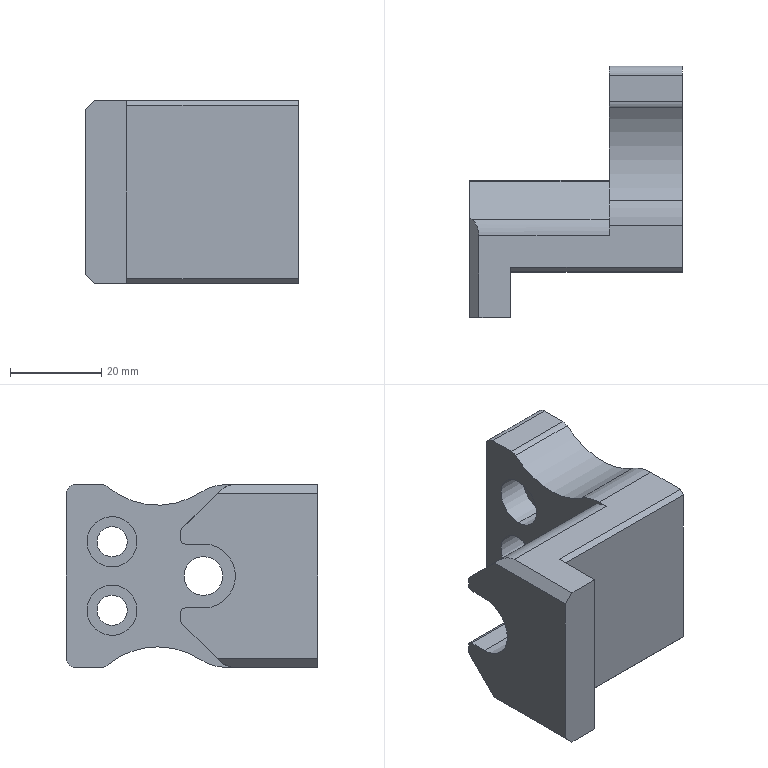Part | SolidWorks | features BaseBody 1 | 1 solid | 55 faces | box 46.5 x 55 x 40 mm | volume 43364 mm3 | cylinder 30 | plane 25 | commonest cylinder face diameters 2 x4 4 x4 6 x4 6.6 x4 11 x4 34 x3